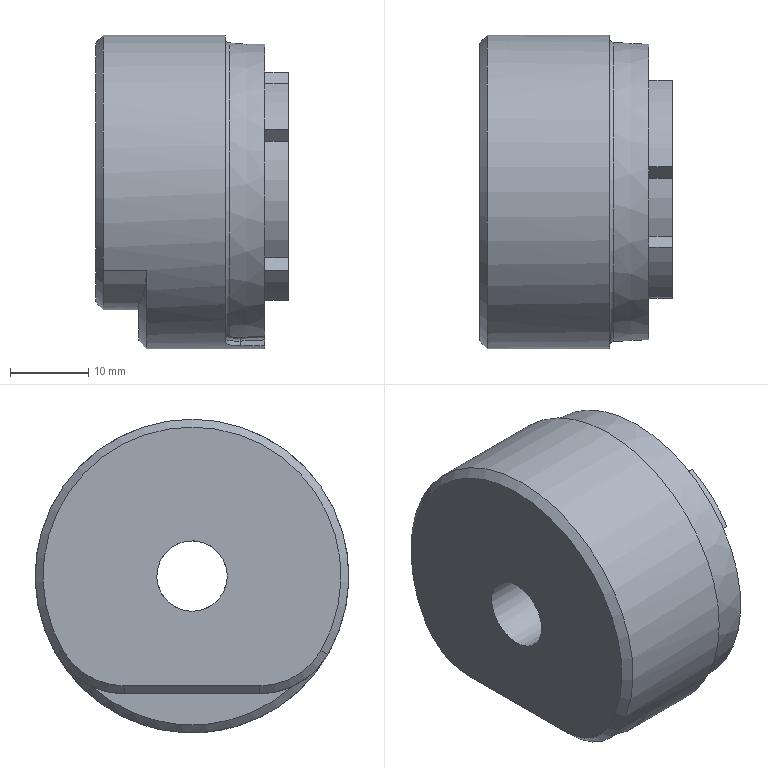Part | STEP file | solid 272 | 1 solid | 43 faces | box 24.594 x 40 x 40 mm | volume 25466 mm3 | plane 18 | cylinder 15 | cone 5 | spline 4 | torus 1 | commonest cylinder face diameters 27.135 x4 31.155 x4 4.02 x2 20 x2 9 x1 14 x1